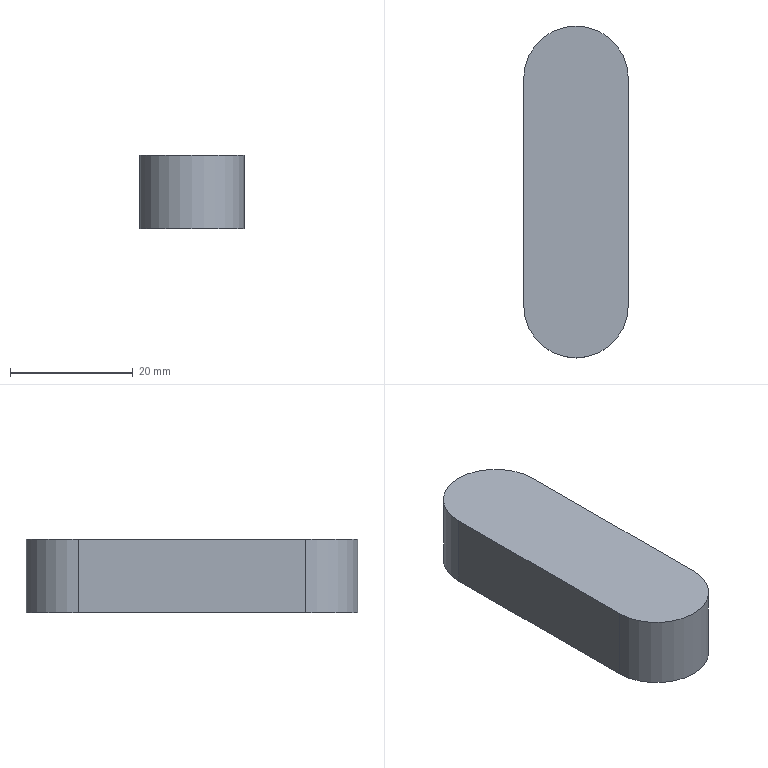Part | NX | features DATUM_CSYS 2, BLEND 1, EXTRUDE 1, SKETCH 1 | 1 solid | 6 faces | box 17 x 54 x 12 mm | volume 10272 mm3 | plane 4 | cylinder 2 | commonest cylinder face diameters 17 x2
STEP:
#1=CARTESIAN_POINT('',(-8.5,18.5,12.));
#2=VERTEX_POINT('',#1);
#3=CARTESIAN_POINT('',(-8.5,-18.5,12.));
#4=VERTEX_POINT('',#3);
#5=CARTESIAN_POINT('',(-8.5,27.,12.));
#6=DIRECTION('',(0.,-1.,0.));
#7=VECTOR('',#6,1000.);
#8=LINE('',#5,#7);
#9=EDGE_CURVE('',#2,#4,#8,.T.);
#10=ORIENTED_EDGE('',*,*,#9,.F.);
#11=CARTESIAN_POINT('',(-8.5,18.5,0.));
#12=VERTEX_POINT('',#11);
#13=CARTESIAN_POINT('',(-8.5,18.5,12.));
#14=DIRECTION('',(0.,0.,-1.));
#15=VECTOR('',#14,1000.);
#16=LINE('',#13,#15);
#17=EDGE_CURVE('',#2,#12,#16,.T.);
#18=ORIENTED_EDGE('',*,*,#17,.T.);
#19=CARTESIAN_POINT('',(-8.5,-18.5,0.));
#20=VERTEX_POINT('',#19);
#21=CARTESIAN_POINT('',(-8.5,27.,0.));
#22=DIRECTION('',(0.,-1.,0.));
#23=VECTOR('',#22,1000.);
#24=LINE('',#21,#23);
#25=EDGE_CURVE('',#12,#20,#24,.T.);
#26=ORIENTED_EDGE('',*,*,#25,.T.);
#27=CARTESIAN_POINT('',(-8.5,-18.5,12.));
#28=DIRECTION('',(0.,0.,-1.));
#29=VECTOR('',#28,1000.);
#30=LINE('',#27,#29);
#31=EDGE_CURVE('',#20,#4,#30,.F.);
#32=ORIENTED_EDGE('',*,*,#31,.T.);
#33=EDGE_LOOP('',(#10,#18,#26,#32));
#34=FACE_BOUND('',#33,.T.);
#35=CARTESIAN_POINT('',(-8.5,27.,12.));
#36=DIRECTION('',(1.,0.,0.));
#37=DIRECTION('',(0.,0.,-1.));
#38=AXIS2_PLACEMENT_3D('',#35,#36,#37);
#39=PLANE('',#38);
#40=ADVANCED_FACE('',(#34),#39,.F.);
#41=CARTESIAN_POINT('',(8.5,-18.5,0.));
#42=VERTEX_POINT('',#41);
#43=CARTESIAN_POINT('',(8.5,18.5,0.));
#44=VERTEX_POINT('',#43);
#45=CARTESIAN_POINT('',(8.5,-27.,0.));
#46=DIRECTION('',(0.,1.,0.));
#47=VECTOR('',#46,1000.);
#48=LINE('',#45,#47);
#49=EDGE_CURVE('',#42,#44,#48,.T.);
#50=ORIENTED_EDGE('',*,*,#49,.T.);
#51=CARTESIAN_POINT('',(8.5,18.5,12.));
#52=VERTEX_POINT('',#51);
#53=CARTESIAN_POINT('',(8.5,18.5,12.));
#54=DIRECTION('',(0.,0.,-1.));
#55=VECTOR('',#54,1000.);
#56=LINE('',#53,#55);
#57=EDGE_CURVE('',#44,#52,#56,.F.);
#58=ORIENTED_EDGE('',*,*,#57,.T.);
#59=CARTESIAN_POINT('',(8.5,-18.5,12.));
#60=VERTEX_POINT('',#59);
#61=CARTESIAN_POINT('',(8.5,-27.,12.));
#62=DIRECTION('',(0.,1.,0.));
#63=VECTOR('',#62,1000.);
#64=LINE('',#61,#63);
#65=EDGE_CURVE('',#60,#52,#64,.T.);
#66=ORIENTED_EDGE('',*,*,#65,.F.);
#67=CARTESIAN_POINT('',(8.5,-18.5,12.));
#68=DIRECTION('',(0.,0.,-1.));
#69=VECTOR('',#68,1000.);
#70=LINE('',#67,#69);
#71=EDGE_CURVE('',#60,#42,#70,.T.);
#72=ORIENTED_EDGE('',*,*,#71,.T.);
#73=EDGE_LOOP('',(#50,#58,#66,#72));
#74=FACE_BOUND('',#73,.T.);
#75=CARTESIAN_POINT('',(8.5,-27.,12.));
#76=DIRECTION('',(-1.,0.,0.));
#77=DIRECTION('',(0.,0.,1.));
#78=AXIS2_PLACEMENT_3D('',#75,#76,#77);
#79=PLANE('',#78);
#80=ADVANCED_FACE('',(#74),#79,.F.);
#81=CARTESIAN_POINT('',(0.,18.5,12.));
#82=DIRECTION('',(0.,0.,1.));
#83=DIRECTION('',(1.,0.,0.));
#84=AXIS2_PLACEMENT_3D('',#81,#82,#83);
#85=CIRCLE('',#84,8.5);
#86=EDGE_CURVE('',#52,#2,#85,.T.);
#87=ORIENTED_EDGE('',*,*,#86,.T.);
#88=ORIENTED_EDGE('',*,*,#9,.T.);
#89=CARTESIAN_POINT('',(0.,-18.5,12.));
#90=DIRECTION('',(0.,0.,1.));
#91=DIRECTION('',(1.,0.,0.));
#92=AXIS2_PLACEMENT_3D('',#89,#90,#91);
#93=CIRCLE('',#92,8.5);
#94=EDGE_CURVE('',#4,#60,#93,.T.);
#95=ORIENTED_EDGE('',*,*,#94,.T.);
#96=ORIENTED_EDGE('',*,*,#65,.T.);
#97=EDGE_LOOP('',(#87,#88,#95,#96));
#98=FACE_BOUND('',#97,.T.);
#99=CARTESIAN_POINT('',(0.,0.,12.));
#100=DIRECTION('',(0.,0.,1.));
#101=DIRECTION('',(1.,0.,0.));
#102=AXIS2_PLACEMENT_3D('',#99,#100,#101);
#103=PLANE('',#102);
#104=ADVANCED_FACE('',(#98),#103,.T.);
#105=ORIENTED_EDGE('',*,*,#25,.F.);
#106=CARTESIAN_POINT('',(0.,18.5,0.));
#107=DIRECTION('',(0.,0.,1.));
#108=DIRECTION('',(1.,0.,0.));
#109=AXIS2_PLACEMENT_3D('',#106,#107,#108);
#110=CIRCLE('',#109,8.5);
#111=EDGE_CURVE('',#12,#44,#110,.F.);
#112=ORIENTED_EDGE('',*,*,#111,.T.);
#113=ORIENTED_EDGE('',*,*,#49,.F.);
#114=CARTESIAN_POINT('',(0.,-18.5,0.));
#115=DIRECTION('',(0.,0.,1.));
#116=DIRECTION('',(1.,0.,0.));
#117=AXIS2_PLACEMENT_3D('',#114,#115,#116);
#118=CIRCLE('',#117,8.5);
#119=EDGE_CURVE('',#42,#20,#118,.F.);
#120=ORIENTED_EDGE('',*,*,#119,.T.);
#121=EDGE_LOOP('',(#105,#112,#113,#120));
#122=FACE_BOUND('',#121,.T.);
#123=CARTESIAN_POINT('',(0.,0.,0.));
#124=DIRECTION('',(0.,0.,1.));
#125=DIRECTION('',(1.,0.,0.));
#126=AXIS2_PLACEMENT_3D('',#123,#124,#125);
#127=PLANE('',#126);
#128=ADVANCED_FACE('',(#122),#127,.F.);
#129=ORIENTED_EDGE('',*,*,#111,.F.);
#130=ORIENTED_EDGE('',*,*,#17,.F.);
#131=ORIENTED_EDGE('',*,*,#86,.F.);
#132=ORIENTED_EDGE('',*,*,#57,.F.);
#133=EDGE_LOOP('',(#129,#130,#131,#132));
#134=FACE_BOUND('',#133,.T.);
#135=CARTESIAN_POINT('',(0.,18.5,12.));
#136=DIRECTION('',(0.,0.,-1.));
#137=DIRECTION('',(-1.,0.,0.));
#138=AXIS2_PLACEMENT_3D('',#135,#136,#137);
#139=CYLINDRICAL_SURFACE('',#138,8.5);
#140=ADVANCED_FACE('',(#134),#139,.T.);
#141=ORIENTED_EDGE('',*,*,#71,.F.);
#142=ORIENTED_EDGE('',*,*,#94,.F.);
#143=ORIENTED_EDGE('',*,*,#31,.F.);
#144=ORIENTED_EDGE('',*,*,#119,.F.);
#145=EDGE_LOOP('',(#141,#142,#143,#144));
#146=FACE_BOUND('',#145,.T.);
#147=CARTESIAN_POINT('',(0.,-18.5,12.));
#148=DIRECTION('',(0.,0.,-1.));
#149=DIRECTION('',(-1.,0.,0.));
#150=AXIS2_PLACEMENT_3D('',#147,#148,#149);
#151=CYLINDRICAL_SURFACE('',#150,8.5);
#152=ADVANCED_FACE('',(#146),#151,.T.);
#153=CLOSED_SHELL('',(#40,#80,#104,#128,#140,#152));
#154=MANIFOLD_SOLID_BREP('',#153);
#155=(LENGTH_UNIT()NAMED_UNIT(*)SI_UNIT(.MILLI.,.METRE.));
#156=UNCERTAINTY_MEASURE_WITH_UNIT(LENGTH_MEASURE(0.00001),#155,'','');
#157=(NAMED_UNIT(*)PLANE_ANGLE_UNIT()SI_UNIT($,.RADIAN.));
#158=(NAMED_UNIT(*)SI_UNIT($,.STERADIAN.)SOLID_ANGLE_UNIT());
#159=(GEOMETRIC_REPRESENTATION_CONTEXT(3)GLOBAL_UNCERTAINTY_ASSIGNED_CONTEXT((#156))GLOBAL_UNIT_ASSIGNED_CONTEXT((#155,#157,#158))REPRESENTATION_CONTEXT('',''));
#160=ADVANCED_BREP_SHAPE_REPRESENTATION('',(#154),#159);